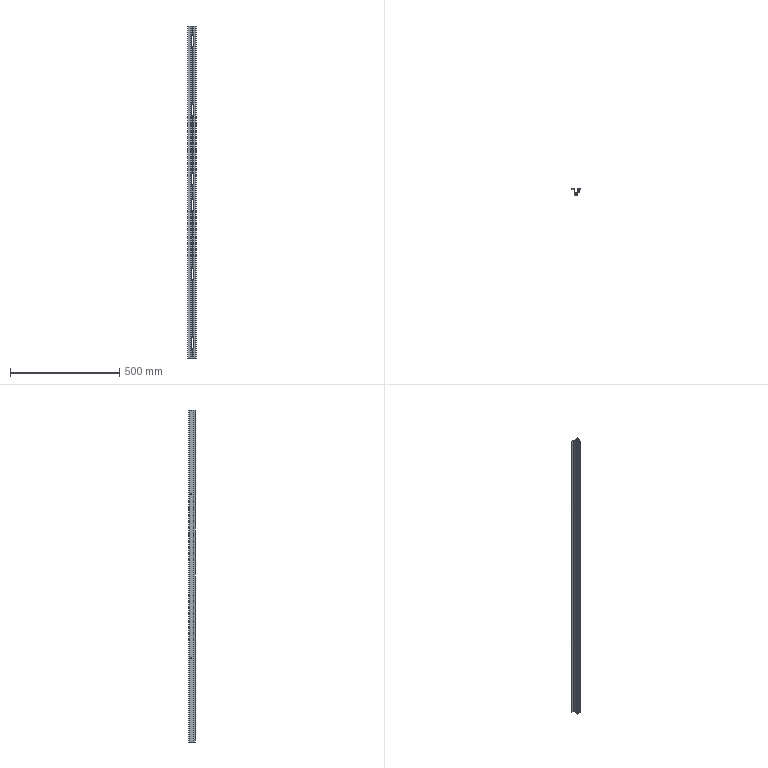Part | SolidWorks | features Emboss 1, Extrusion 1, ICE 1 | 1 solid | 102 faces | box 40 x 29.5 x 1520 mm | volume 285493 mm3 | plane 65 | cylinder 37 | commonest cylinder face diameters 9 x30 2 x5 3 x2